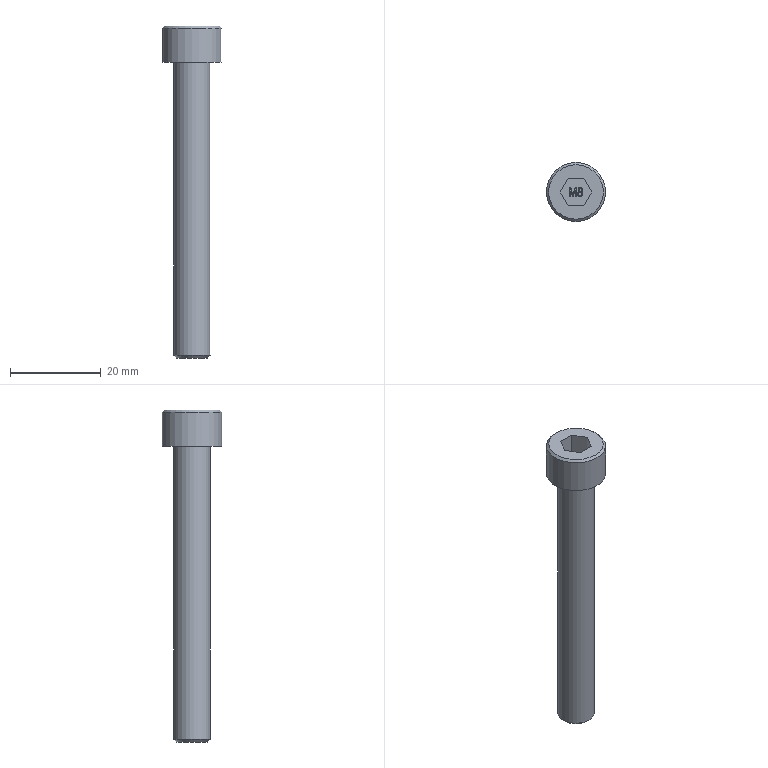Part | STEP file | EM10806500 | 1 solid | 38 faces | box 13 x 13 x 73 mm | volume 4164 mm3 | plane 25 | other 9 | cylinder 2 | cone 2 | commonest cylinder face diameters 8 x1 13 x1